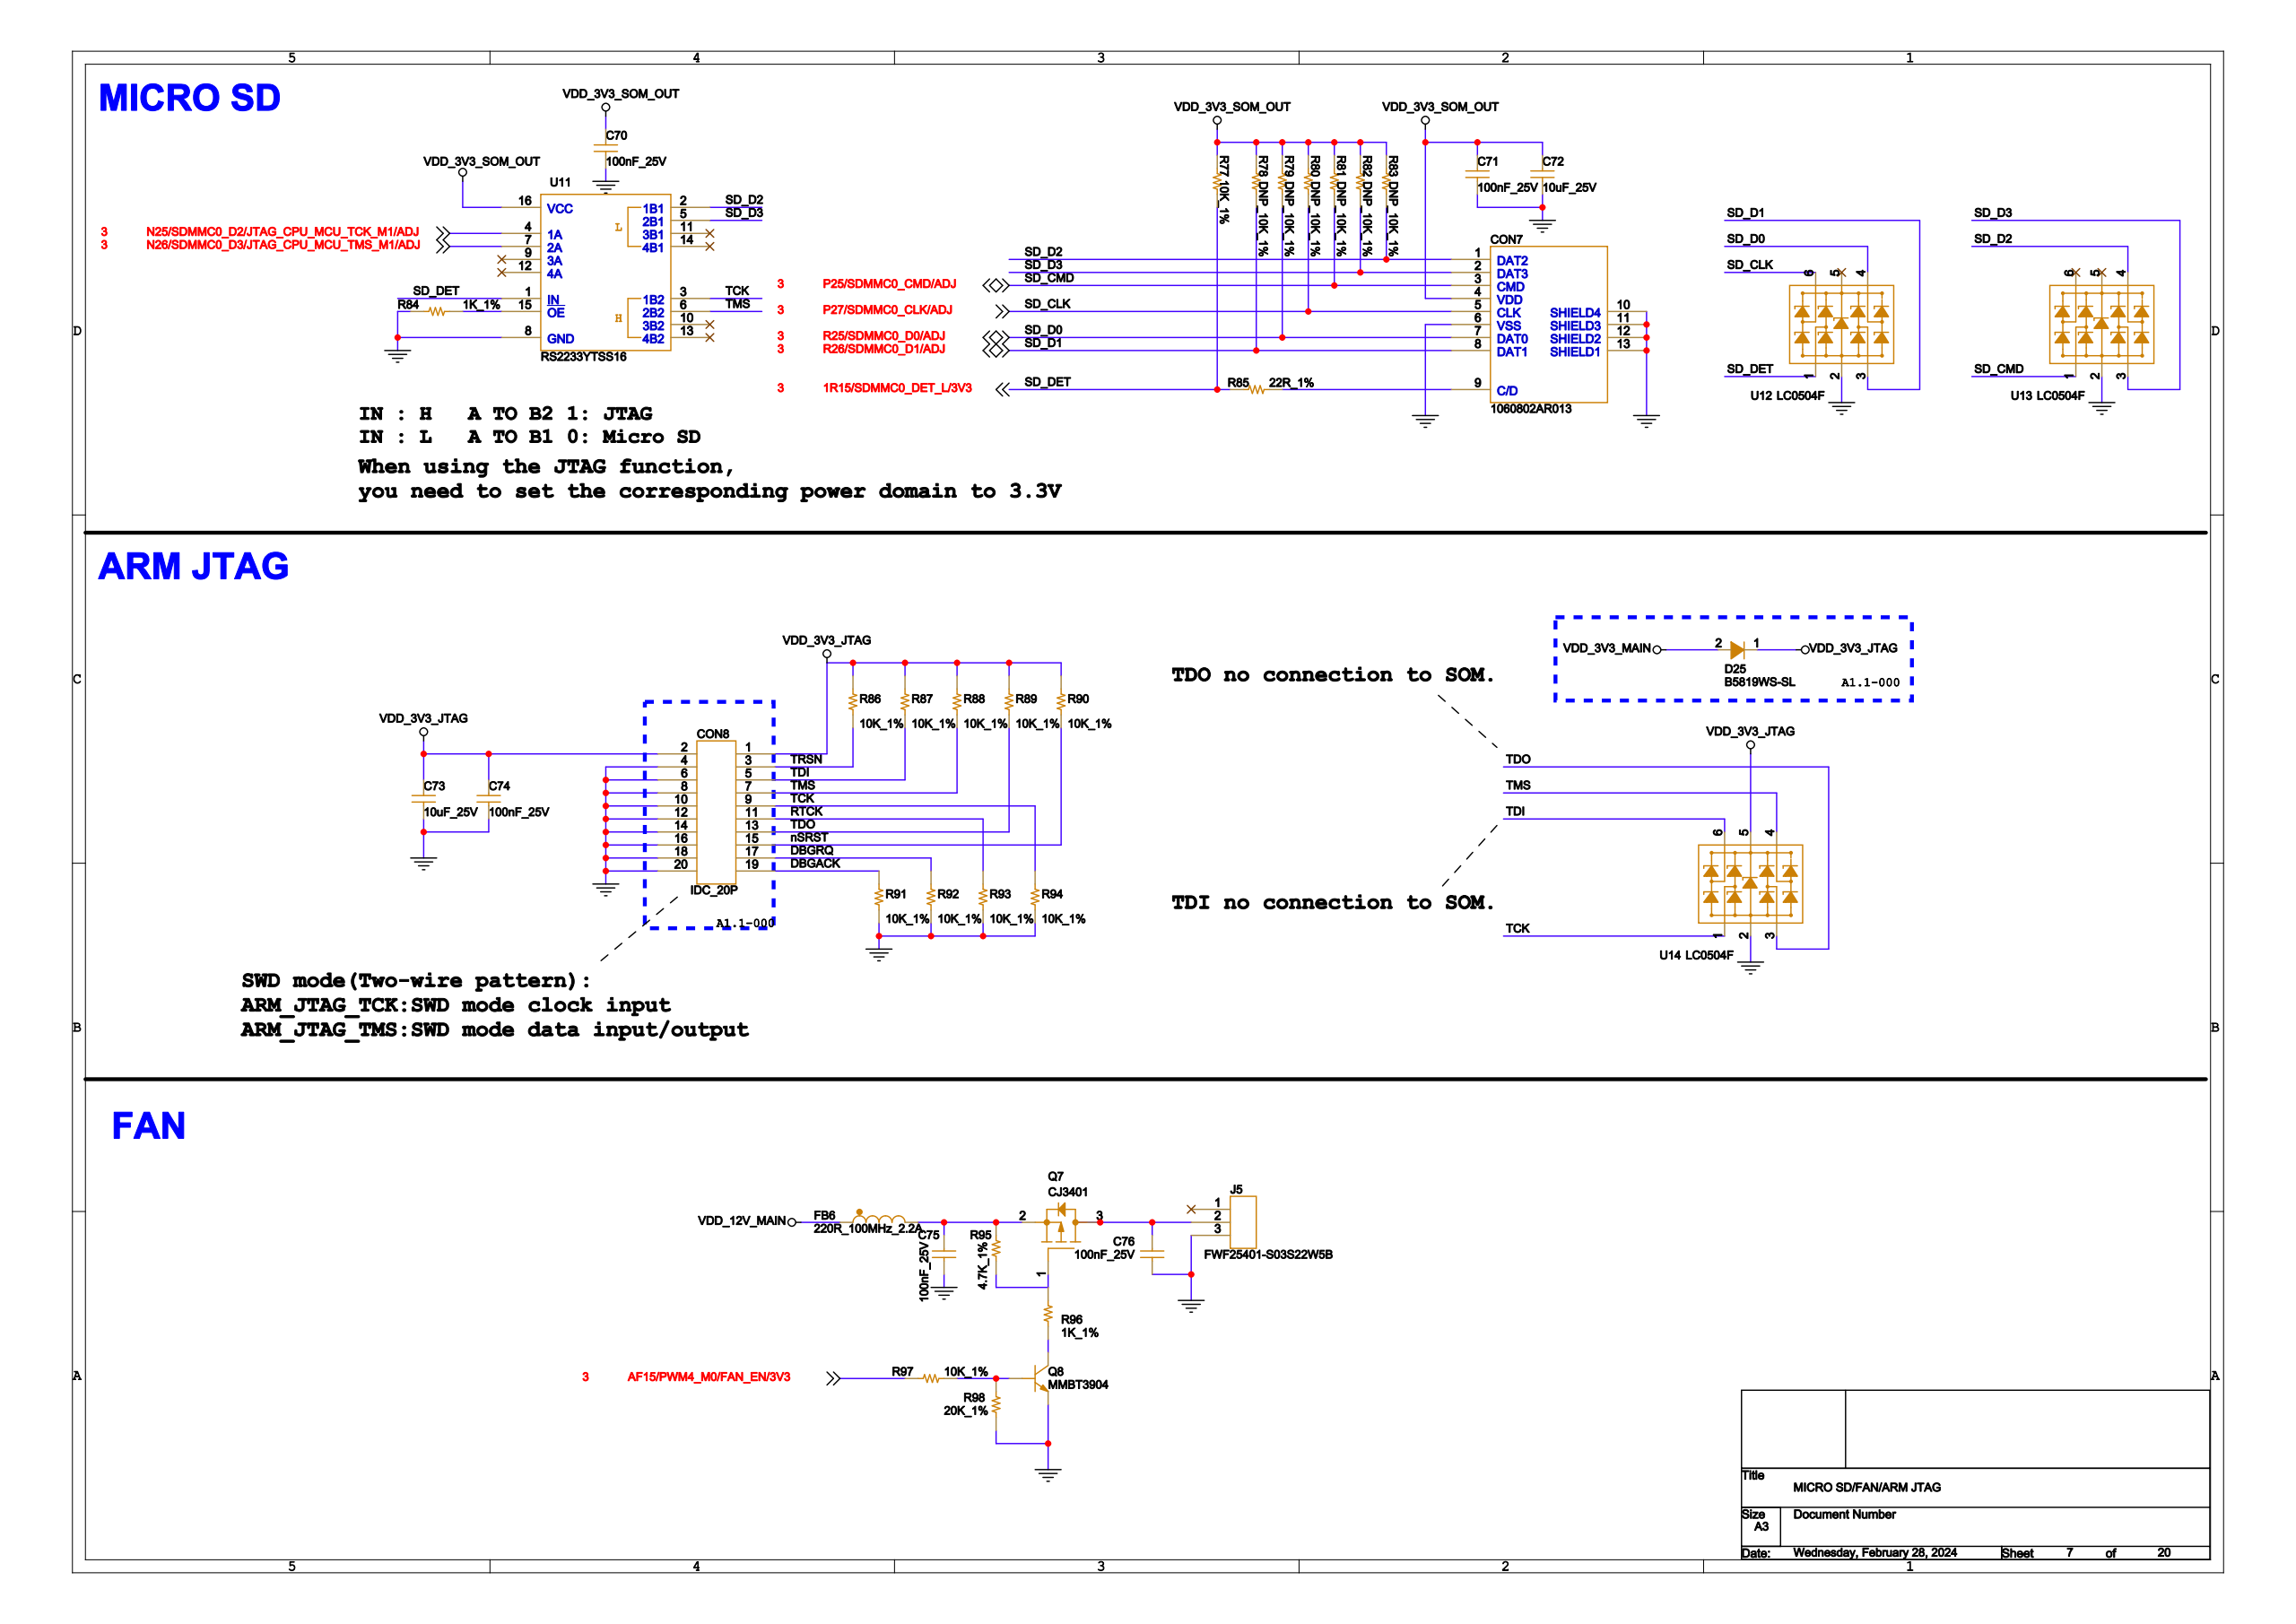Circuit board | Cadence Allegro | 1024 parts | 682 nets | one sheet of the schematic
Parts on this sheet (reference | value | footprint):
C70 | 100nF_25V | C0402
C71 | 100nF_25V | C0402
C72 | 10uF_25V | C0603
C73 | 10uF_25V | C0603
C74 | 100nF_25V | C0402
C76 | 100nF_25V | C0402
CON7 | 1060802AR013 | CON_TF_CARD
CON8 | IDC_20P | CON_2D54_2X10_TH_BOX_90
D25 | B5819WS-SL | SOD-323
FB6 | 220R_100MHz_2A | L0603
J5 | FWF25401-S03S22W5B | MOL22-23-2031
Q7 | CJ3401 | SOT23-3
Q8 | MMBT3904 | SOT23-3_DBZ3
R77 | 10K_1% | R0402
R78 | DNP_10K_1% | R0402
R79 | DNP_10K_1% | R0402
R80 | DNP_10K_1% | R0402
R81 | DNP_10K_1% | R0402
R82 | DNP_10K_1% | R0402
R83 | DNP_10K_1% | R0402
R84 | 1K_1% | R0402
R85 | 22R_1% | R0402
R86 | 10K_1% | R0402
R87 | 10K_1% | R0402
R88 | 10K_1% | R0402
R89 | 10K_1% | R0402
R90 | 10K_1% | R0402
R91 | 10K_1% | R0402
R92 | 10K_1% | R0402
R93 | 10K_1% | R0402
R94 | 10K_1% | R0402
R96 | 1K_1% | R0402
R97 | 10K_1% | R0402
R98 | 20K_1% | R0402
U11 | RS2233YTSS16 | TSSOP16
U12 | LC0504F | SOT363
U13 | LC0504F | SOT363
U14 | LC0504F | SOT363
Nets of these parts (net: part-pin ...):
VDD_3V3_JTAG: C73-1 C74-1 CON8-1 CON8-2 D25-1 R86-1 R87-1 R88-1 R89-1 R90-1 U14-5
GND: C70-2 C71-2 C72-2 C73-2 C74-2 C76-2 CON7-6 CON7-10 CON7-11 CON7-12 CON7-13 CON8-4 CON8-6 CON8-8 CON8-10 CON8-12 CON8-14 CON8-16 CON8-18 CON8-20 J5-3 Q8-2 R84-2 R91-2 R92-2 R93-2 R94-2 R98-2 U11-8 U12-2 U13-2 U14-2
RTCK: CON8-11 R93-1
TDO: CON8-13 R89-2 U14-3
NSRST: CON8-15 R90-2
DBGRQ: CON8-17 R92-1
DBGACK: CON8-19 R91-1
TRSN: CON8-3 R86-2
TDI: CON8-5 R87-2 U14-6
TMS: CON8-7 R88-2 U11-6 U14-4
TCK: CON8-9 R94-1 U11-3 U14-1
VDD_3V3_MAIN: D25-2
AF15/PWM4_M0/FAN_EN/3V3: R97-1
1R15/SDMMC0_DET_L/3V3: R77-2 R85-1 U11-1 U12-1
P27/SDMMC0_CLK/ADJ: CON7-5 R80-2 U12-6
N26/SDMMC0_D3/JTAG_CPU_MCU_TMS_: U11-7
R26/SDMMC0_D1/ADJ: CON7-8 R78-2 U12-3
R25/SDMMC0_D0/ADJ: CON7-7 R79-2 U12-4
P25/SDMMC0_CMD/ADJ: CON7-3 R81-2 U13-1
N25/SDMMC0_D2/JTAG_CPU_MCU_TCK_: U11-4
VDD_3V3_SOM_OUT: C70-1 C71-1 C72-1 CON7-4 R77-1 R78-1 R79-1 R80-1 R81-1 R82-1 R83-1 U11-16
N21588963: R84-1 U11-15
N21587752: Q7-1 R96-1
N21587836: Q8-3 R96-2
VDD_12V_MAIN: FB6-1
N21587779: FB6-2 Q7-2
N21587770: Q8-1 R97-2 R98-1
SD_D2: CON7-1 R83-2 U11-2 U13-4
SD_D3: CON7-2 R82-2 U11-5 U13-3
N21589141: CON7-9 R85-2
N21587766: C76-1 J5-2 Q7-3